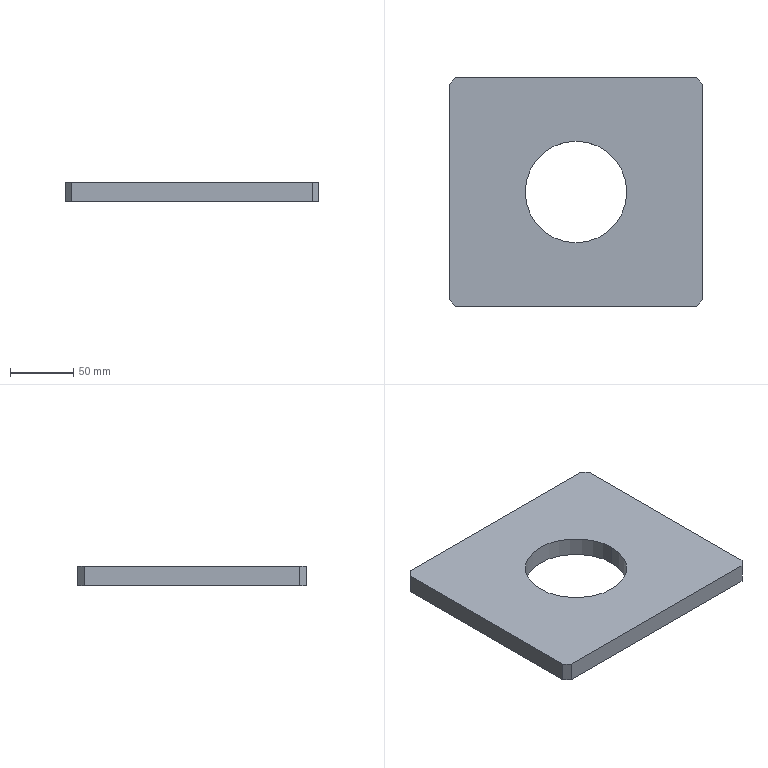Part | STEP file | 001-009-Riveting mechanism electric cylinder spacer block | 1 solid | 12 faces | box 200 x 180 x 15 mm | volume 463852 mm3 | plane 10 | cylinder 2 | commonest cylinder face diameters 80 x2
STEP:
#1=CARTESIAN_POINT('',(0.,0.,0.));
#2=DIRECTION('',(0.,0.,1.));
#3=DIRECTION('',(1.,0.,0.));
#4=AXIS2_PLACEMENT_3D('',#1,#2,#3);
#5=CARTESIAN_POINT('',(40.,0.,0.));
#6=VERTEX_POINT('',#5);
#7=CARTESIAN_POINT('',(40.,0.,15.));
#8=VERTEX_POINT('',#7);
#9=CARTESIAN_POINT('',(40.,0.,0.));
#10=DIRECTION('',(0.,0.,1.));
#11=VECTOR('',#10,1.);
#12=LINE('',#9,#11);
#13=CARTESIAN_POINT('',(0.,0.,0.));
#14=DIRECTION('',(0.,0.,1.));
#15=DIRECTION('',(1.,0.,0.));
#16=AXIS2_PLACEMENT_3D('',#13,#14,#15);
#17=CYLINDRICAL_SURFACE('',#16,40.);
#18=CARTESIAN_POINT('',(6.283,0.));
#19=DIRECTION('',(0.,1.));
#20=VECTOR('',#19,1.);
#21=LINE('',#18,#20);
#22=(GEOMETRIC_REPRESENTATION_CONTEXT(2)PARAMETRIC_REPRESENTATION_CONTEXT()REPRESENTATION_CONTEXT('',''));
#23=DEFINITIONAL_REPRESENTATION('',(#21),#22);
#24=PCURVE('',#17,#23);
#25=CARTESIAN_POINT('',(0.,0.,0.));
#26=DIRECTION('',(0.,0.,1.));
#27=DIRECTION('',(1.,0.,0.));
#28=AXIS2_PLACEMENT_3D('',#25,#26,#27);
#29=CYLINDRICAL_SURFACE('',#28,40.);
#30=CARTESIAN_POINT('',(0.,0.));
#31=DIRECTION('',(0.,1.));
#32=VECTOR('',#31,1.);
#33=LINE('',#30,#32);
#34=(GEOMETRIC_REPRESENTATION_CONTEXT(2)PARAMETRIC_REPRESENTATION_CONTEXT()REPRESENTATION_CONTEXT('',''));
#35=DEFINITIONAL_REPRESENTATION('',(#33),#34);
#36=PCURVE('',#29,#35);
#37=SURFACE_CURVE('',#12,(#24,#36),.PCURVE_S1.);
#38=EDGE_CURVE('',#6,#8,#37,.T.);
#39=ORIENTED_EDGE('',*,*,#38,.T.);
#40=CARTESIAN_POINT('',(-40.,0.,15.));
#41=VERTEX_POINT('',#40);
#42=CARTESIAN_POINT('',(0.,0.,15.));
#43=DIRECTION('',(0.,0.,1.));
#44=DIRECTION('',(1.,0.,0.));
#45=AXIS2_PLACEMENT_3D('',#42,#43,#44);
#46=CIRCLE('',#45,40.);
#47=CARTESIAN_POINT('',(0.,15.));
#48=DIRECTION('',(1.,0.));
#49=VECTOR('',#48,1.);
#50=LINE('',#47,#49);
#51=(GEOMETRIC_REPRESENTATION_CONTEXT(2)PARAMETRIC_REPRESENTATION_CONTEXT()REPRESENTATION_CONTEXT('',''));
#52=DEFINITIONAL_REPRESENTATION('',(#50),#51);
#53=PCURVE('',#17,#52);
#54=CARTESIAN_POINT('',(0.,0.,15.));
#55=DIRECTION('',(0.,0.,-1.));
#56=DIRECTION('',(-1.,0.,0.));
#57=AXIS2_PLACEMENT_3D('',#54,#55,#56);
#58=PLANE('',#57);
#59=CARTESIAN_POINT('',(-40.,0.));
#60=CARTESIAN_POINT('',(-40.,69.282));
#61=CARTESIAN_POINT('',(20.,34.641));
#62=CARTESIAN_POINT('',(80.,0.));
#63=CARTESIAN_POINT('',(20.,-34.641));
#64=CARTESIAN_POINT('',(-40.,-69.282));
#65=CARTESIAN_POINT('',(-40.,0.));
#66=(BOUNDED_CURVE()B_SPLINE_CURVE(2,(#59,#60,#61,#62,#63,#64,#65),.UNSPECIFIED.,.T.,.F.)B_SPLINE_CURVE_WITH_KNOTS((1,2,2,2,2,1),(-2.094,0.,2.094,4.189,6.283,8.378),.UNSPECIFIED.)CURVE()GEOMETRIC_REPRESENTATION_ITEM()RATIONAL_B_SPLINE_CURVE((1.,0.5,1.,0.5,1.,0.5,1.))REPRESENTATION_ITEM(''));
#67=(GEOMETRIC_REPRESENTATION_CONTEXT(2)PARAMETRIC_REPRESENTATION_CONTEXT()REPRESENTATION_CONTEXT('',''));
#68=DEFINITIONAL_REPRESENTATION('',(#66),#67);
#69=PCURVE('',#58,#68);
#70=SURFACE_CURVE('',#46,(#53,#69),.PCURVE_S1.);
#71=EDGE_CURVE('',#41,#8,#70,.T.);
#72=ORIENTED_EDGE('',*,*,#71,.F.);
#73=CARTESIAN_POINT('',(-40.,0.,0.));
#74=VERTEX_POINT('',#73);
#75=CARTESIAN_POINT('',(-40.,0.,0.));
#76=DIRECTION('',(0.,0.,1.));
#77=VECTOR('',#76,1.);
#78=LINE('',#75,#77);
#79=CARTESIAN_POINT('',(3.142,0.));
#80=DIRECTION('',(0.,1.));
#81=VECTOR('',#80,1.);
#82=LINE('',#79,#81);
#83=(GEOMETRIC_REPRESENTATION_CONTEXT(2)PARAMETRIC_REPRESENTATION_CONTEXT()REPRESENTATION_CONTEXT('',''));
#84=DEFINITIONAL_REPRESENTATION('',(#82),#83);
#85=PCURVE('',#17,#84);
#86=CARTESIAN_POINT('',(3.142,0.));
#87=DIRECTION('',(0.,1.));
#88=VECTOR('',#87,1.);
#89=LINE('',#86,#88);
#90=(GEOMETRIC_REPRESENTATION_CONTEXT(2)PARAMETRIC_REPRESENTATION_CONTEXT()REPRESENTATION_CONTEXT('',''));
#91=DEFINITIONAL_REPRESENTATION('',(#89),#90);
#92=PCURVE('',#29,#91);
#93=SURFACE_CURVE('',#78,(#85,#92),.PCURVE_S1.);
#94=EDGE_CURVE('',#74,#41,#93,.T.);
#95=ORIENTED_EDGE('',*,*,#94,.F.);
#96=CARTESIAN_POINT('',(0.,0.,0.));
#97=DIRECTION('',(0.,0.,1.));
#98=DIRECTION('',(1.,0.,0.));
#99=AXIS2_PLACEMENT_3D('',#96,#97,#98);
#100=CIRCLE('',#99,40.);
#101=CARTESIAN_POINT('',(0.,0.));
#102=DIRECTION('',(1.,0.));
#103=VECTOR('',#102,1.);
#104=LINE('',#101,#103);
#105=(GEOMETRIC_REPRESENTATION_CONTEXT(2)PARAMETRIC_REPRESENTATION_CONTEXT()REPRESENTATION_CONTEXT('',''));
#106=DEFINITIONAL_REPRESENTATION('',(#104),#105);
#107=PCURVE('',#17,#106);
#108=CARTESIAN_POINT('',(0.,0.,0.));
#109=DIRECTION('',(0.,0.,-1.));
#110=DIRECTION('',(-1.,0.,0.));
#111=AXIS2_PLACEMENT_3D('',#108,#109,#110);
#112=PLANE('',#111);
#113=CARTESIAN_POINT('',(-40.,0.));
#114=CARTESIAN_POINT('',(-40.,69.282));
#115=CARTESIAN_POINT('',(20.,34.641));
#116=CARTESIAN_POINT('',(80.,0.));
#117=CARTESIAN_POINT('',(20.,-34.641));
#118=CARTESIAN_POINT('',(-40.,-69.282));
#119=CARTESIAN_POINT('',(-40.,0.));
#120=(BOUNDED_CURVE()B_SPLINE_CURVE(2,(#113,#114,#115,#116,#117,#118,#119),.UNSPECIFIED.,.T.,.F.)B_SPLINE_CURVE_WITH_KNOTS((1,2,2,2,2,1),(-2.094,0.,2.094,4.189,6.283,8.378),.UNSPECIFIED.)CURVE()GEOMETRIC_REPRESENTATION_ITEM()RATIONAL_B_SPLINE_CURVE((1.,0.5,1.,0.5,1.,0.5,1.))REPRESENTATION_ITEM(''));
#121=(GEOMETRIC_REPRESENTATION_CONTEXT(2)PARAMETRIC_REPRESENTATION_CONTEXT()REPRESENTATION_CONTEXT('',''));
#122=DEFINITIONAL_REPRESENTATION('',(#120),#121);
#123=PCURVE('',#112,#122);
#124=SURFACE_CURVE('',#100,(#107,#123),.PCURVE_S1.);
#125=EDGE_CURVE('',#74,#6,#124,.T.);
#126=ORIENTED_EDGE('',*,*,#125,.T.);
#127=EDGE_LOOP('',(#39,#72,#95,#126));
#128=FACE_BOUND('',#127,.F.);
#129=ADVANCED_FACE('',(#128),#17,.F.);
#130=CARTESIAN_POINT('',(100.,-85.,15.));
#131=VERTEX_POINT('',#130);
#132=CARTESIAN_POINT('',(100.,85.,15.));
#133=VERTEX_POINT('',#132);
#134=CARTESIAN_POINT('',(100.,-90.,15.));
#135=DIRECTION('',(0.,1.,0.));
#136=VECTOR('',#135,1.);
#137=LINE('',#134,#136);
#138=CARTESIAN_POINT('',(100.,-90.,15.));
#139=DIRECTION('',(-1.,0.,0.));
#140=DIRECTION('',(0.,-1.,0.));
#141=AXIS2_PLACEMENT_3D('',#138,#139,#140);
#142=PLANE('',#141);
#143=CARTESIAN_POINT('',(0.,0.));
#144=DIRECTION('',(-1.,0.));
#145=VECTOR('',#144,1.);
#146=LINE('',#143,#145);
#147=(GEOMETRIC_REPRESENTATION_CONTEXT(2)PARAMETRIC_REPRESENTATION_CONTEXT()REPRESENTATION_CONTEXT('',''));
#148=DEFINITIONAL_REPRESENTATION('',(#146),#147);
#149=PCURVE('',#142,#148);
#150=CARTESIAN_POINT('',(-100.,-90.));
#151=DIRECTION('',(0.,1.));
#152=VECTOR('',#151,1.);
#153=LINE('',#150,#152);
#154=(GEOMETRIC_REPRESENTATION_CONTEXT(2)PARAMETRIC_REPRESENTATION_CONTEXT()REPRESENTATION_CONTEXT('',''));
#155=DEFINITIONAL_REPRESENTATION('',(#153),#154);
#156=PCURVE('',#58,#155);
#157=SURFACE_CURVE('',#137,(#149,#156),.PCURVE_S1.);
#158=EDGE_CURVE('',#131,#133,#157,.T.);
#159=ORIENTED_EDGE('',*,*,#158,.F.);
#160=CARTESIAN_POINT('',(100.,-85.,0.));
#161=VERTEX_POINT('',#160);
#162=CARTESIAN_POINT('',(100.,-85.,15.));
#163=DIRECTION('',(0.,0.,-1.));
#164=VECTOR('',#163,1.);
#165=LINE('',#162,#164);
#166=CARTESIAN_POINT('',(-5.,0.));
#167=DIRECTION('',(0.,-1.));
#168=VECTOR('',#167,1.);
#169=LINE('',#166,#168);
#170=(GEOMETRIC_REPRESENTATION_CONTEXT(2)PARAMETRIC_REPRESENTATION_CONTEXT()REPRESENTATION_CONTEXT('',''));
#171=DEFINITIONAL_REPRESENTATION('',(#169),#170);
#172=PCURVE('',#142,#171);
#173=CARTESIAN_POINT('',(100.,-85.,15.));
#174=DIRECTION('',(-0.7071,0.7071,0.));
#175=DIRECTION('',(0.,0.,-1.));
#176=AXIS2_PLACEMENT_3D('',#173,#174,#175);
#177=PLANE('',#176);
#178=CARTESIAN_POINT('',(0.,0.));
#179=DIRECTION('',(1.,0.));
#180=VECTOR('',#179,1.);
#181=LINE('',#178,#180);
#182=(GEOMETRIC_REPRESENTATION_CONTEXT(2)PARAMETRIC_REPRESENTATION_CONTEXT()REPRESENTATION_CONTEXT('',''));
#183=DEFINITIONAL_REPRESENTATION('',(#181),#182);
#184=PCURVE('',#177,#183);
#185=SURFACE_CURVE('',#165,(#172,#184),.PCURVE_S1.);
#186=EDGE_CURVE('',#131,#161,#185,.T.);
#187=ORIENTED_EDGE('',*,*,#186,.T.);
#188=CARTESIAN_POINT('',(100.,85.,0.));
#189=VERTEX_POINT('',#188);
#190=CARTESIAN_POINT('',(100.,-90.,0.));
#191=DIRECTION('',(0.,1.,0.));
#192=VECTOR('',#191,1.);
#193=LINE('',#190,#192);
#194=CARTESIAN_POINT('',(0.,-15.));
#195=DIRECTION('',(-1.,0.));
#196=VECTOR('',#195,1.);
#197=LINE('',#194,#196);
#198=(GEOMETRIC_REPRESENTATION_CONTEXT(2)PARAMETRIC_REPRESENTATION_CONTEXT()REPRESENTATION_CONTEXT('',''));
#199=DEFINITIONAL_REPRESENTATION('',(#197),#198);
#200=PCURVE('',#142,#199);
#201=CARTESIAN_POINT('',(-100.,-90.));
#202=DIRECTION('',(0.,1.));
#203=VECTOR('',#202,1.);
#204=LINE('',#201,#203);
#205=(GEOMETRIC_REPRESENTATION_CONTEXT(2)PARAMETRIC_REPRESENTATION_CONTEXT()REPRESENTATION_CONTEXT('',''));
#206=DEFINITIONAL_REPRESENTATION('',(#204),#205);
#207=PCURVE('',#112,#206);
#208=SURFACE_CURVE('',#193,(#200,#207),.PCURVE_S1.);
#209=EDGE_CURVE('',#161,#189,#208,.T.);
#210=ORIENTED_EDGE('',*,*,#209,.T.);
#211=CARTESIAN_POINT('',(100.,85.,15.));
#212=DIRECTION('',(0.,0.,1.));
#213=VECTOR('',#212,1.);
#214=LINE('',#211,#213);
#215=CARTESIAN_POINT('',(-175.,0.));
#216=DIRECTION('',(0.,1.));
#217=VECTOR('',#216,1.);
#218=LINE('',#215,#217);
#219=(GEOMETRIC_REPRESENTATION_CONTEXT(2)PARAMETRIC_REPRESENTATION_CONTEXT()REPRESENTATION_CONTEXT('',''));
#220=DEFINITIONAL_REPRESENTATION('',(#218),#219);
#221=PCURVE('',#142,#220);
#222=CARTESIAN_POINT('',(95.,90.,15.));
#223=DIRECTION('',(-0.7071,-0.7071,0.));
#224=DIRECTION('',(0.,0.,-1.));
#225=AXIS2_PLACEMENT_3D('',#222,#223,#224);
#226=PLANE('',#225);
#227=CARTESIAN_POINT('',(0.,7.071));
#228=DIRECTION('',(-1.,0.));
#229=VECTOR('',#228,1.);
#230=LINE('',#227,#229);
#231=(GEOMETRIC_REPRESENTATION_CONTEXT(2)PARAMETRIC_REPRESENTATION_CONTEXT()REPRESENTATION_CONTEXT('',''));
#232=DEFINITIONAL_REPRESENTATION('',(#230),#231);
#233=PCURVE('',#226,#232);
#234=SURFACE_CURVE('',#214,(#221,#233),.PCURVE_S1.);
#235=EDGE_CURVE('',#189,#133,#234,.T.);
#236=ORIENTED_EDGE('',*,*,#235,.T.);
#237=EDGE_LOOP('',(#159,#187,#210,#236));
#238=FACE_BOUND('',#237,.T.);
#239=ADVANCED_FACE('',(#238),#142,.F.);
#240=CARTESIAN_POINT('',(95.,90.,0.));
#241=VERTEX_POINT('',#240);
#242=CARTESIAN_POINT('',(-95.,90.,0.));
#243=VERTEX_POINT('',#242);
#244=CARTESIAN_POINT('',(-100.,90.,0.));
#245=DIRECTION('',(-1.,0.,0.));
#246=VECTOR('',#245,1.);
#247=LINE('',#244,#246);
#248=CARTESIAN_POINT('',(-100.,90.,15.));
#249=DIRECTION('',(0.,-1.,0.));
#250=DIRECTION('',(0.,0.,-1.));
#251=AXIS2_PLACEMENT_3D('',#248,#249,#250);
#252=PLANE('',#251);
#253=CARTESIAN_POINT('',(15.,0.));
#254=DIRECTION('',(0.,-1.));
#255=VECTOR('',#254,1.);
#256=LINE('',#253,#255);
#257=(GEOMETRIC_REPRESENTATION_CONTEXT(2)PARAMETRIC_REPRESENTATION_CONTEXT()REPRESENTATION_CONTEXT('',''));
#258=DEFINITIONAL_REPRESENTATION('',(#256),#257);
#259=PCURVE('',#252,#258);
#260=CARTESIAN_POINT('',(100.,90.));
#261=DIRECTION('',(1.,0.));
#262=VECTOR('',#261,1.);
#263=LINE('',#260,#262);
#264=(GEOMETRIC_REPRESENTATION_CONTEXT(2)PARAMETRIC_REPRESENTATION_CONTEXT()REPRESENTATION_CONTEXT('',''));
#265=DEFINITIONAL_REPRESENTATION('',(#263),#264);
#266=PCURVE('',#112,#265);
#267=SURFACE_CURVE('',#247,(#259,#266),.PCURVE_S1.);
#268=EDGE_CURVE('',#241,#243,#267,.T.);
#269=ORIENTED_EDGE('',*,*,#268,.T.);
#270=CARTESIAN_POINT('',(-95.,90.,15.));
#271=VERTEX_POINT('',#270);
#272=CARTESIAN_POINT('',(-95.,90.,15.));
#273=DIRECTION('',(0.,0.,1.));
#274=VECTOR('',#273,1.);
#275=LINE('',#272,#274);
#276=CARTESIAN_POINT('',(0.,5.));
#277=DIRECTION('',(-1.,0.));
#278=VECTOR('',#277,1.);
#279=LINE('',#276,#278);
#280=(GEOMETRIC_REPRESENTATION_CONTEXT(2)PARAMETRIC_REPRESENTATION_CONTEXT()REPRESENTATION_CONTEXT('',''));
#281=DEFINITIONAL_REPRESENTATION('',(#279),#280);
#282=PCURVE('',#252,#281);
#283=CARTESIAN_POINT('',(-100.,85.,15.));
#284=DIRECTION('',(0.7071,-0.7071,0.));
#285=DIRECTION('',(0.,0.,-1.));
#286=AXIS2_PLACEMENT_3D('',#283,#284,#285);
#287=PLANE('',#286);
#288=CARTESIAN_POINT('',(0.,7.071));
#289=DIRECTION('',(-1.,0.));
#290=VECTOR('',#289,1.);
#291=LINE('',#288,#290);
#292=(GEOMETRIC_REPRESENTATION_CONTEXT(2)PARAMETRIC_REPRESENTATION_CONTEXT()REPRESENTATION_CONTEXT('',''));
#293=DEFINITIONAL_REPRESENTATION('',(#291),#292);
#294=PCURVE('',#287,#293);
#295=SURFACE_CURVE('',#275,(#282,#294),.PCURVE_S1.);
#296=EDGE_CURVE('',#243,#271,#295,.T.);
#297=ORIENTED_EDGE('',*,*,#296,.T.);
#298=CARTESIAN_POINT('',(95.,90.,15.));
#299=VERTEX_POINT('',#298);
#300=CARTESIAN_POINT('',(-100.,90.,15.));
#301=DIRECTION('',(-1.,0.,0.));
#302=VECTOR('',#301,1.);
#303=LINE('',#300,#302);
#304=CARTESIAN_POINT('',(0.,0.));
#305=DIRECTION('',(0.,-1.));
#306=VECTOR('',#305,1.);
#307=LINE('',#304,#306);
#308=(GEOMETRIC_REPRESENTATION_CONTEXT(2)PARAMETRIC_REPRESENTATION_CONTEXT()REPRESENTATION_CONTEXT('',''));
#309=DEFINITIONAL_REPRESENTATION('',(#307),#308);
#310=PCURVE('',#252,#309);
#311=CARTESIAN_POINT('',(100.,90.));
#312=DIRECTION('',(1.,0.));
#313=VECTOR('',#312,1.);
#314=LINE('',#311,#313);
#315=(GEOMETRIC_REPRESENTATION_CONTEXT(2)PARAMETRIC_REPRESENTATION_CONTEXT()REPRESENTATION_CONTEXT('',''));
#316=DEFINITIONAL_REPRESENTATION('',(#314),#315);
#317=PCURVE('',#58,#316);
#318=SURFACE_CURVE('',#303,(#310,#317),.PCURVE_S1.);
#319=EDGE_CURVE('',#299,#271,#318,.T.);
#320=ORIENTED_EDGE('',*,*,#319,.F.);
#321=CARTESIAN_POINT('',(95.,90.,15.));
#322=DIRECTION('',(0.,0.,-1.));
#323=VECTOR('',#322,1.);
#324=LINE('',#321,#323);
#325=CARTESIAN_POINT('',(0.,195.));
#326=DIRECTION('',(1.,0.));
#327=VECTOR('',#326,1.);
#328=LINE('',#325,#327);
#329=(GEOMETRIC_REPRESENTATION_CONTEXT(2)PARAMETRIC_REPRESENTATION_CONTEXT()REPRESENTATION_CONTEXT('',''));
#330=DEFINITIONAL_REPRESENTATION('',(#328),#329);
#331=PCURVE('',#252,#330);
#332=CARTESIAN_POINT('',(0.,0.));
#333=DIRECTION('',(1.,0.));
#334=VECTOR('',#333,1.);
#335=LINE('',#332,#334);
#336=(GEOMETRIC_REPRESENTATION_CONTEXT(2)PARAMETRIC_REPRESENTATION_CONTEXT()REPRESENTATION_CONTEXT('',''));
#337=DEFINITIONAL_REPRESENTATION('',(#335),#336);
#338=PCURVE('',#226,#337);
#339=SURFACE_CURVE('',#324,(#331,#338),.PCURVE_S1.);
#340=EDGE_CURVE('',#299,#241,#339,.T.);
#341=ORIENTED_EDGE('',*,*,#340,.T.);
#342=EDGE_LOOP('',(#269,#297,#320,#341));
#343=FACE_BOUND('',#342,.T.);
#344=ADVANCED_FACE('',(#343),#252,.F.);
#345=CARTESIAN_POINT('',(-100.,85.,0.));
#346=VERTEX_POINT('',#345);
#347=CARTESIAN_POINT('',(-100.,-85.,0.));
#348=VERTEX_POINT('',#347);
#349=CARTESIAN_POINT('',(-100.,-90.,0.));
#350=DIRECTION('',(0.,-1.,0.));
#351=VECTOR('',#350,1.);
#352=LINE('',#349,#351);
#353=CARTESIAN_POINT('',(-100.,-90.,15.));
#354=DIRECTION('',(1.,0.,0.));
#355=DIRECTION('',(0.,0.,-1.));
#356=AXIS2_PLACEMENT_3D('',#353,#354,#355);
#357=PLANE('',#356);
#358=CARTESIAN_POINT('',(15.,0.));
#359=DIRECTION('',(0.,-1.));
#360=VECTOR('',#359,1.);
#361=LINE('',#358,#360);
#362=(GEOMETRIC_REPRESENTATION_CONTEXT(2)PARAMETRIC_REPRESENTATION_CONTEXT()REPRESENTATION_CONTEXT('',''));
#363=DEFINITIONAL_REPRESENTATION('',(#361),#362);
#364=PCURVE('',#357,#363);
#365=CARTESIAN_POINT('',(100.,-90.));
#366=DIRECTION('',(0.,-1.));
#367=VECTOR('',#366,1.);
#368=LINE('',#365,#367);
#369=(GEOMETRIC_REPRESENTATION_CONTEXT(2)PARAMETRIC_REPRESENTATION_CONTEXT()REPRESENTATION_CONTEXT('',''));
#370=DEFINITIONAL_REPRESENTATION('',(#368),#369);
#371=PCURVE('',#112,#370);
#372=SURFACE_CURVE('',#352,(#364,#371),.PCURVE_S1.);
#373=EDGE_CURVE('',#346,#348,#372,.T.);
#374=ORIENTED_EDGE('',*,*,#373,.T.);
#375=CARTESIAN_POINT('',(-100.,-85.,15.));
#376=VERTEX_POINT('',#375);
#377=CARTESIAN_POINT('',(-100.,-85.,15.));
#378=DIRECTION('',(0.,0.,1.));
#379=VECTOR('',#378,1.);
#380=LINE('',#377,#379);
#381=CARTESIAN_POINT('',(0.,5.));
#382=DIRECTION('',(-1.,0.));
#383=VECTOR('',#382,1.);
#384=LINE('',#381,#383);
#385=(GEOMETRIC_REPRESENTATION_CONTEXT(2)PARAMETRIC_REPRESENTATION_CONTEXT()REPRESENTATION_CONTEXT('',''));
#386=DEFINITIONAL_REPRESENTATION('',(#384),#385);
#387=PCURVE('',#357,#386);
#388=CARTESIAN_POINT('',(-95.,-90.,15.));
#389=DIRECTION('',(0.7071,0.7071,0.));
#390=DIRECTION('',(0.,0.,-1.));
#391=AXIS2_PLACEMENT_3D('',#388,#389,#390);
#392=PLANE('',#391);
#393=CARTESIAN_POINT('',(0.,7.071));
#394=DIRECTION('',(-1.,0.));
#395=VECTOR('',#394,1.);
#396=LINE('',#393,#395);
#397=(GEOMETRIC_REPRESENTATION_CONTEXT(2)PARAMETRIC_REPRESENTATION_CONTEXT()REPRESENTATION_CONTEXT('',''));
#398=DEFINITIONAL_REPRESENTATION('',(#396),#397);
#399=PCURVE('',#392,#398);
#400=SURFACE_CURVE('',#380,(#387,#399),.PCURVE_S1.);
#401=EDGE_CURVE('',#348,#376,#400,.T.);
#402=ORIENTED_EDGE('',*,*,#401,.T.);
#403=CARTESIAN_POINT('',(-100.,85.,15.));
#404=VERTEX_POINT('',#403);
#405=CARTESIAN_POINT('',(-100.,-90.,15.));
#406=DIRECTION('',(0.,-1.,0.));
#407=VECTOR('',#406,1.);
#408=LINE('',#405,#407);
#409=CARTESIAN_POINT('',(0.,0.));
#410=DIRECTION('',(0.,-1.));
#411=VECTOR('',#410,1.);
#412=LINE('',#409,#411);
#413=(GEOMETRIC_REPRESENTATION_CONTEXT(2)PARAMETRIC_REPRESENTATION_CONTEXT()REPRESENTATION_CONTEXT('',''));
#414=DEFINITIONAL_REPRESENTATION('',(#412),#413);
#415=PCURVE('',#357,#414);
#416=CARTESIAN_POINT('',(100.,-90.));
#417=DIRECTION('',(0.,-1.));
#418=VECTOR('',#417,1.);
#419=LINE('',#416,#418);
#420=(GEOMETRIC_REPRESENTATION_CONTEXT(2)PARAMETRIC_REPRESENTATION_CONTEXT()REPRESENTATION_CONTEXT('',''));
#421=DEFINITIONAL_REPRESENTATION('',(#419),#420);
#422=PCURVE('',#58,#421);
#423=SURFACE_CURVE('',#408,(#415,#422),.PCURVE_S1.);
#424=EDGE_CURVE('',#404,#376,#423,.T.);
#425=ORIENTED_EDGE('',*,*,#424,.F.);
#426=CARTESIAN_POINT('',(-100.,85.,15.));
#427=DIRECTION('',(0.,0.,-1.));
#428=VECTOR('',#427,1.);
#429=LINE('',#426,#428);
#430=CARTESIAN_POINT('',(0.,175.));
#431=DIRECTION('',(1.,0.));
#432=VECTOR('',#431,1.);
#433=LINE('',#430,#432);
#434=(GEOMETRIC_REPRESENTATION_CONTEXT(2)PARAMETRIC_REPRESENTATION_CONTEXT()REPRESENTATION_CONTEXT('',''));
#435=DEFINITIONAL_REPRESENTATION('',(#433),#434);
#436=PCURVE('',#357,#435);
#437=CARTESIAN_POINT('',(0.,0.));
#438=DIRECTION('',(1.,0.));
#439=VECTOR('',#438,1.);
#440=LINE('',#437,#439);
#441=(GEOMETRIC_REPRESENTATION_CONTEXT(2)PARAMETRIC_REPRESENTATION_CONTEXT()REPRESENTATION_CONTEXT('',''));
#442=DEFINITIONAL_REPRESENTATION('',(#440),#441);
#443=PCURVE('',#287,#442);
#444=SURFACE_CURVE('',#429,(#436,#443),.PCURVE_S1.);
#445=EDGE_CURVE('',#404,#346,#444,.T.);
#446=ORIENTED_EDGE('',*,*,#445,.T.);
#447=EDGE_LOOP('',(#374,#402,#425,#446));
#448=FACE_BOUND('',#447,.T.);
#449=ADVANCED_FACE('',(#448),#357,.F.);
#450=CARTESIAN_POINT('',(-95.,-90.,0.));
#451=VERTEX_POINT('',#450);
#452=CARTESIAN_POINT('',(95.,-90.,0.));
#453=VERTEX_POINT('',#452);
#454=CARTESIAN_POINT('',(-100.,-90.,0.));
#455=DIRECTION('',(1.,0.,0.));
#456=VECTOR('',#455,1.);
#457=LINE('',#454,#456);
#458=CARTESIAN_POINT('',(-100.,-90.,15.));
#459=DIRECTION('',(0.,1.,0.));
#460=DIRECTION('',(0.,0.,1.));
#461=AXIS2_PLACEMENT_3D('',#458,#459,#460);
#462=PLANE('',#461);
#463=CARTESIAN_POINT('',(-15.,0.));
#464=DIRECTION('',(0.,1.));
#465=VECTOR('',#464,1.);
#466=LINE('',#463,#465);
#467=(GEOMETRIC_REPRESENTATION_CONTEXT(2)PARAMETRIC_REPRESENTATION_CONTEXT()REPRESENTATION_CONTEXT('',''));
#468=DEFINITIONAL_REPRESENTATION('',(#466),#467);
#469=PCURVE('',#462,#468);
#470=CARTESIAN_POINT('',(100.,-90.));
#471=DIRECTION('',(-1.,0.));
#472=VECTOR('',#471,1.);
#473=LINE('',#470,#472);
#474=(GEOMETRIC_REPRESENTATION_CONTEXT(2)PARAMETRIC_REPRESENTATION_CONTEXT()REPRESENTATION_CONTEXT('',''));
#475=DEFINITIONAL_REPRESENTATION('',(#473),#474);
#476=PCURVE('',#112,#475);
#477=SURFACE_CURVE('',#457,(#469,#476),.PCURVE_S1.);
#478=EDGE_CURVE('',#451,#453,#477,.T.);
#479=ORIENTED_EDGE('',*,*,#478,.T.);
#480=CARTESIAN_POINT('',(95.,-90.,15.));
#481=VERTEX_POINT('',#480);
#482=CARTESIAN_POINT('',(95.,-90.,15.));
#483=DIRECTION('',(0.,0.,1.));
#484=VECTOR('',#483,1.);
#485=LINE('',#482,#484);
#486=CARTESIAN_POINT('',(0.,195.));
#487=DIRECTION('',(1.,0.));
#488=VECTOR('',#487,1.);
#489=LINE('',#486,#488);
#490=(GEOMETRIC_REPRESENTATION_CONTEXT(2)PARAMETRIC_REPRESENTATION_CONTEXT()REPRESENTATION_CONTEXT('',''));
#491=DEFINITIONAL_REPRESENTATION('',(#489),#490);
#492=PCURVE('',#462,#491);
#493=CARTESIAN_POINT('',(0.,7.071));
#494=DIRECTION('',(-1.,0.));
#495=VECTOR('',#494,1.);
#496=LINE('',#493,#495);
#497=(GEOMETRIC_REPRESENTATION_CONTEXT(2)PARAMETRIC_REPRESENTATION_CONTEXT()REPRESENTATION_CONTEXT('',''));
#498=DEFINITIONAL_REPRESENTATION('',(#496),#497);
#499=PCURVE('',#177,#498);
#500=SURFACE_CURVE('',#485,(#492,#499),.PCURVE_S1.);
#501=EDGE_CURVE('',#453,#481,#500,.T.);
#502=ORIENTED_EDGE('',*,*,#501,.T.);
#503=CARTESIAN_POINT('',(-95.,-90.,15.));
#504=VERTEX_POINT('',#503);
#505=CARTESIAN_POINT('',(-100.,-90.,15.));
#506=DIRECTION('',(1.,0.,0.));
#507=VECTOR('',#506,1.);
#508=LINE('',#505,#507);
#509=CARTESIAN_POINT('',(0.,0.));
#510=DIRECTION('',(0.,1.));
#511=VECTOR('',#510,1.);
#512=LINE('',#509,#511);
#513=(GEOMETRIC_REPRESENTATION_CONTEXT(2)PARAMETRIC_REPRESENTATION_CONTEXT()REPRESENTATION_CONTEXT('',''));
#514=DEFINITIONAL_REPRESENTATION('',(#512),#513);
#515=PCURVE('',#462,#514);
#516=CARTESIAN_POINT('',(100.,-90.));
#517=DIRECTION('',(-1.,0.));
#518=VECTOR('',#517,1.);
#519=LINE('',#516,#518);
#520=(GEOMETRIC_REPRESENTATION_CONTEXT(2)PARAMETRIC_REPRESENTATION_CONTEXT()REPRESENTATION_CONTEXT('',''));
#521=DEFINITIONAL_REPRESENTATION('',(#519),#520);
#522=PCURVE('',#58,#521);
#523=SURFACE_CURVE('',#508,(#515,#522),.PCURVE_S1.);
#524=EDGE_CURVE('',#504,#481,#523,.T.);
#525=ORIENTED_EDGE('',*,*,#524,.F.);
#526=CARTESIAN_POINT('',(-95.,-90.,15.));
#527=DIRECTION('',(0.,0.,-1.));
#528=VECTOR('',#527,1.);
#529=LINE('',#526,#528);
#530=CARTESIAN_POINT('',(0.,5.));
#531=DIRECTION('',(-1.,0.));
#532=VECTOR('',#531,1.);
#533=LINE('',#530,#532);
#534=(GEOMETRIC_REPRESENTATION_CONTEXT(2)PARAMETRIC_REPRESENTATION_CONTEXT()REPRESENTATION_CONTEXT('',''));
#535=DEFINITIONAL_REPRESENTATION('',(#533),#534);
#536=PCURVE('',#462,#535);
#537=CARTESIAN_POINT('',(0.,0.));
#538=DIRECTION('',(1.,0.));
#539=VECTOR('',#538,1.);
#540=LINE('',#537,#539);
#541=(GEOMETRIC_REPRESENTATION_CONTEXT(2)PARAMETRIC_REPRESENTATION_CONTEXT()REPRESENTATION_CONTEXT('',''));
#542=DEFINITIONAL_REPRESENTATION('',(#540),#541);
#543=PCURVE('',#392,#542);
#544=SURFACE_CURVE('',#529,(#536,#543),.PCURVE_S1.);
#545=EDGE_CURVE('',#504,#451,#544,.T.);
#546=ORIENTED_EDGE('',*,*,#545,.T.);
#547=EDGE_LOOP('',(#479,#502,#525,#546));
#548=FACE_BOUND('',#547,.T.);
#549=ADVANCED_FACE('',(#548),#462,.F.);
#550=CARTESIAN_POINT('',(0.,0.,15.));
#551=DIRECTION('',(0.,0.,1.));
#552=DIRECTION('',(1.,0.,0.));
#553=AXIS2_PLACEMENT_3D('',#550,#551,#552);
#554=CIRCLE('',#553,40.);
#555=CARTESIAN_POINT('',(-40.,0.));
#556=CARTESIAN_POINT('',(-40.,69.282));
#557=CARTESIAN_POINT('',(20.,34.641));
#558=CARTESIAN_POINT('',(80.,0.));
#559=CARTESIAN_POINT('',(20.,-34.641));
#560=CARTESIAN_POINT('',(-40.,-69.282));
#561=CARTESIAN_POINT('',(-40.,0.));
#562=(BOUNDED_CURVE()B_SPLINE_CURVE(2,(#555,#556,#557,#558,#559,#560,#561),.UNSPECIFIED.,.T.,.F.)B_SPLINE_CURVE_WITH_KNOTS((1,2,2,2,2,1),(-2.094,0.,2.094,4.189,6.283,8.378),.UNSPECIFIED.)CURVE()GEOMETRIC_REPRESENTATION_ITEM()RATIONAL_B_SPLINE_CURVE((1.,0.5,1.,0.5,1.,0.5,1.))REPRESENTATION_ITEM(''));
#563=(GEOMETRIC_REPRESENTATION_CONTEXT(2)PARAMETRIC_REPRESENTATION_CONTEXT()REPRESENTATION_CONTEXT('',''));
#564=DEFINITIONAL_REPRESENTATION('',(#562),#563);
#565=PCURVE('',#58,#564);
#566=CARTESIAN_POINT('',(0.,15.));
#567=DIRECTION('',(1.,0.));
#568=VECTOR('',#567,1.);
#569=LINE('',#566,#568);
#570=(GEOMETRIC_REPRESENTATION_CONTEXT(2)PARAMETRIC_REPRESENTATION_CONTEXT()REPRESENTATION_CONTEXT('',''));
#571=DEFINITIONAL_REPRESENTATION('',(#569),#570);
#572=PCURVE('',#29,#571);
#573=SURFACE_CURVE('',#554,(#565,#572),.PCURVE_S1.);
#574=EDGE_CURVE('',#8,#41,#573,.T.);
#575=ORIENTED_EDGE('',*,*,#574,.F.);
#576=ORIENTED_EDGE('',*,*,#71,.F.);
#577=EDGE_LOOP('',(#575,#576));
#578=FACE_BOUND('',#577,.T.);
#579=ORIENTED_EDGE('',*,*,#524,.T.);
#580=CARTESIAN_POINT('',(100.,-85.,15.));
#581=DIRECTION('',(0.7071,0.7071,0.));
#582=VECTOR('',#581,1.);
#583=LINE('',#580,#582);
#584=CARTESIAN_POINT('',(-100.,-85.));
#585=DIRECTION('',(-0.7071,0.7071));
#586=VECTOR('',#585,1.);
#587=LINE('',#584,#586);
#588=(GEOMETRIC_REPRESENTATION_CONTEXT(2)PARAMETRIC_REPRESENTATION_CONTEXT()REPRESENTATION_CONTEXT('',''));
#589=DEFINITIONAL_REPRESENTATION('',(#587),#588);
#590=PCURVE('',#58,#589);
#591=CARTESIAN_POINT('',(0.,0.));
#592=DIRECTION('',(0.,-1.));
#593=VECTOR('',#592,1.);
#594=LINE('',#591,#593);
#595=(GEOMETRIC_REPRESENTATION_CONTEXT(2)PARAMETRIC_REPRESENTATION_CONTEXT()REPRESENTATION_CONTEXT('',''));
#596=DEFINITIONAL_REPRESENTATION('',(#594),#595);
#597=PCURVE('',#177,#596);
#598=SURFACE_CURVE('',#583,(#590,#597),.PCURVE_S1.);
#599=EDGE_CURVE('',#481,#131,#598,.T.);
#600=ORIENTED_EDGE('',*,*,#599,.T.);
#601=ORIENTED_EDGE('',*,*,#158,.T.);
#602=CARTESIAN_POINT('',(95.,90.,15.));
#603=DIRECTION('',(-0.7071,0.7071,0.));
#604=VECTOR('',#603,1.);
#605=LINE('',#602,#604);
#606=CARTESIAN_POINT('',(-95.,90.));
#607=DIRECTION('',(0.7071,0.7071));
#608=VECTOR('',#607,1.);
#609=LINE('',#606,#608);
#610=(GEOMETRIC_REPRESENTATION_CONTEXT(2)PARAMETRIC_REPRESENTATION_CONTEXT()REPRESENTATION_CONTEXT('',''));
#611=DEFINITIONAL_REPRESENTATION('',(#609),#610);
#612=PCURVE('',#58,#611);
#613=CARTESIAN_POINT('',(0.,0.));
#614=DIRECTION('',(0.,-1.));
#615=VECTOR('',#614,1.);
#616=LINE('',#613,#615);
#617=(GEOMETRIC_REPRESENTATION_CONTEXT(2)PARAMETRIC_REPRESENTATION_CONTEXT()REPRESENTATION_CONTEXT('',''));
#618=DEFINITIONAL_REPRESENTATION('',(#616),#617);
#619=PCURVE('',#226,#618);
#620=SURFACE_CURVE('',#605,(#612,#619),.PCURVE_S1.);
#621=EDGE_CURVE('',#133,#299,#620,.T.);
#622=ORIENTED_EDGE('',*,*,#621,.T.);
#623=ORIENTED_EDGE('',*,*,#319,.T.);
#624=CARTESIAN_POINT('',(-100.,85.,15.));
#625=DIRECTION('',(-0.7071,-0.7071,0.));
#626=VECTOR('',#625,1.);
#627=LINE('',#624,#626);
#628=CARTESIAN_POINT('',(100.,85.));
#629=DIRECTION('',(0.7071,-0.7071));
#630=VECTOR('',#629,1.);
#631=LINE('',#628,#630);
#632=(GEOMETRIC_REPRESENTATION_CONTEXT(2)PARAMETRIC_REPRESENTATION_CONTEXT()REPRESENTATION_CONTEXT('',''));
#633=DEFINITIONAL_REPRESENTATION('',(#631),#632);
#634=PCURVE('',#58,#633);
#635=CARTESIAN_POINT('',(0.,0.));
#636=DIRECTION('',(0.,-1.));
#637=VECTOR('',#636,1.);
#638=LINE('',#635,#637);
#639=(GEOMETRIC_REPRESENTATION_CONTEXT(2)PARAMETRIC_REPRESENTATION_CONTEXT()REPRESENTATION_CONTEXT('',''));
#640=DEFINITIONAL_REPRESENTATION('',(#638),#639);
#641=PCURVE('',#287,#640);
#642=SURFACE_CURVE('',#627,(#634,#641),.PCURVE_S1.);
#643=EDGE_CURVE('',#271,#404,#642,.T.);
#644=ORIENTED_EDGE('',*,*,#643,.T.);
#645=ORIENTED_EDGE('',*,*,#424,.T.);
#646=CARTESIAN_POINT('',(-95.,-90.,15.));
#647=DIRECTION('',(0.7071,-0.7071,0.));
#648=VECTOR('',#647,1.);
#649=LINE('',#646,#648);
#650=CARTESIAN_POINT('',(95.,-90.));
#651=DIRECTION('',(-0.7071,-0.7071));
#652=VECTOR('',#651,1.);
#653=LINE('',#650,#652);
#654=(GEOMETRIC_REPRESENTATION_CONTEXT(2)PARAMETRIC_REPRESENTATION_CONTEXT()REPRESENTATION_CONTEXT('',''));
#655=DEFINITIONAL_REPRESENTATION('',(#653),#654);
#656=PCURVE('',#58,#655);
#657=CARTESIAN_POINT('',(0.,0.));
#658=DIRECTION('',(0.,-1.));
#659=VECTOR('',#658,1.);
#660=LINE('',#657,#659);
#661=(GEOMETRIC_REPRESENTATION_CONTEXT(2)PARAMETRIC_REPRESENTATION_CONTEXT()REPRESENTATION_CONTEXT('',''));
#662=DEFINITIONAL_REPRESENTATION('',(#660),#661);
#663=PCURVE('',#392,#662);
#664=SURFACE_CURVE('',#649,(#656,#663),.PCURVE_S1.);
#665=EDGE_CURVE('',#376,#504,#664,.T.);
#666=ORIENTED_EDGE('',*,*,#665,.T.);
#667=EDGE_LOOP('',(#579,#600,#601,#622,#623,#644,#645,#666));
#668=FACE_BOUND('',#667,.T.);
#669=ADVANCED_FACE('',(#578,#668),#58,.F.);
#670=CARTESIAN_POINT('',(0.,0.,0.));
#671=DIRECTION('',(0.,0.,1.));
#672=DIRECTION('',(1.,0.,0.));
#673=AXIS2_PLACEMENT_3D('',#670,#671,#672);
#674=CIRCLE('',#673,40.);
#675=CARTESIAN_POINT('',(-40.,0.));
#676=CARTESIAN_POINT('',(-40.,69.282));
#677=CARTESIAN_POINT('',(20.,34.641));
#678=CARTESIAN_POINT('',(80.,0.));
#679=CARTESIAN_POINT('',(20.,-34.641));
#680=CARTESIAN_POINT('',(-40.,-69.282));
#681=CARTESIAN_POINT('',(-40.,0.));
#682=(BOUNDED_CURVE()B_SPLINE_CURVE(2,(#675,#676,#677,#678,#679,#680,#681),.UNSPECIFIED.,.T.,.F.)B_SPLINE_CURVE_WITH_KNOTS((1,2,2,2,2,1),(-2.094,0.,2.094,4.189,6.283,8.378),.UNSPECIFIED.)CURVE()GEOMETRIC_REPRESENTATION_ITEM()RATIONAL_B_SPLINE_CURVE((1.,0.5,1.,0.5,1.,0.5,1.))REPRESENTATION_ITEM(''));
#683=(GEOMETRIC_REPRESENTATION_CONTEXT(2)PARAMETRIC_REPRESENTATION_CONTEXT()REPRESENTATION_CONTEXT('',''));
#684=DEFINITIONAL_REPRESENTATION('',(#682),#683);
#685=PCURVE('',#112,#684);
#686=CARTESIAN_POINT('',(0.,0.));
#687=DIRECTION('',(1.,0.));
#688=VECTOR('',#687,1.);
#689=LINE('',#686,#688);
#690=(GEOMETRIC_REPRESENTATION_CONTEXT(2)PARAMETRIC_REPRESENTATION_CONTEXT()REPRESENTATION_CONTEXT('',''));
#691=DEFINITIONAL_REPRESENTATION('',(#689),#690);
#692=PCURVE('',#29,#691);
#693=SURFACE_CURVE('',#674,(#685,#692),.PCURVE_S1.);
#694=EDGE_CURVE('',#6,#74,#693,.T.);
#695=ORIENTED_EDGE('',*,*,#694,.T.);
#696=ORIENTED_EDGE('',*,*,#125,.T.);
#697=EDGE_LOOP('',(#695,#696));
#698=FACE_BOUND('',#697,.T.);
#699=ORIENTED_EDGE('',*,*,#209,.F.);
#700=CARTESIAN_POINT('',(92.5,-92.5,0.));
#701=DIRECTION('',(-0.7071,-0.7071,0.));
#702=VECTOR('',#701,1.);
#703=LINE('',#700,#702);
#704=CARTESIAN_POINT('',(-92.5,-92.5));
#705=DIRECTION('',(0.7071,-0.7071));
#706=VECTOR('',#705,1.);
#707=LINE('',#704,#706);
#708=(GEOMETRIC_REPRESENTATION_CONTEXT(2)PARAMETRIC_REPRESENTATION_CONTEXT()REPRESENTATION_CONTEXT('',''));
#709=DEFINITIONAL_REPRESENTATION('',(#707),#708);
#710=PCURVE('',#112,#709);
#711=CARTESIAN_POINT('',(15.,10.607));
#712=DIRECTION('',(0.,1.));
#713=VECTOR('',#712,1.);
#714=LINE('',#711,#713);
#715=(GEOMETRIC_REPRESENTATION_CONTEXT(2)PARAMETRIC_REPRESENTATION_CONTEXT()REPRESENTATION_CONTEXT('',''));
#716=DEFINITIONAL_REPRESENTATION('',(#714),#715);
#717=PCURVE('',#177,#716);
#718=SURFACE_CURVE('',#703,(#710,#717),.PCURVE_S1.);
#719=EDGE_CURVE('',#161,#453,#718,.T.);
#720=ORIENTED_EDGE('',*,*,#719,.T.);
#721=ORIENTED_EDGE('',*,*,#478,.F.);
#722=CARTESIAN_POINT('',(-92.5,-92.5,0.));
#723=DIRECTION('',(-0.7071,0.7071,0.));
#724=VECTOR('',#723,1.);
#725=LINE('',#722,#724);
#726=CARTESIAN_POINT('',(92.5,-92.5));
#727=DIRECTION('',(0.7071,0.7071));
#728=VECTOR('',#727,1.);
#729=LINE('',#726,#728);
#730=(GEOMETRIC_REPRESENTATION_CONTEXT(2)PARAMETRIC_REPRESENTATION_CONTEXT()REPRESENTATION_CONTEXT('',''));
#731=DEFINITIONAL_REPRESENTATION('',(#729),#730);
#732=PCURVE('',#112,#731);
#733=CARTESIAN_POINT('',(15.,-3.536));
#734=DIRECTION('',(0.,1.));
#735=VECTOR('',#734,1.);
#736=LINE('',#733,#735);
#737=(GEOMETRIC_REPRESENTATION_CONTEXT(2)PARAMETRIC_REPRESENTATION_CONTEXT()REPRESENTATION_CONTEXT('',''));
#738=DEFINITIONAL_REPRESENTATION('',(#736),#737);
#739=PCURVE('',#392,#738);
#740=SURFACE_CURVE('',#725,(#732,#739),.PCURVE_S1.);
#741=EDGE_CURVE('',#451,#348,#740,.T.);
#742=ORIENTED_EDGE('',*,*,#741,.T.);
#743=ORIENTED_EDGE('',*,*,#373,.F.);
#744=CARTESIAN_POINT('',(-92.5,92.5,0.));
#745=DIRECTION('',(0.7071,0.7071,0.));
#746=VECTOR('',#745,1.);
#747=LINE('',#744,#746);
#748=CARTESIAN_POINT('',(92.5,92.5));
#749=DIRECTION('',(-0.7071,0.7071));
#750=VECTOR('',#749,1.);
#751=LINE('',#748,#750);
#752=(GEOMETRIC_REPRESENTATION_CONTEXT(2)PARAMETRIC_REPRESENTATION_CONTEXT()REPRESENTATION_CONTEXT('',''));
#753=DEFINITIONAL_REPRESENTATION('',(#751),#752);
#754=PCURVE('',#112,#753);
#755=CARTESIAN_POINT('',(15.,10.607));
#756=DIRECTION('',(0.,1.));
#757=VECTOR('',#756,1.);
#758=LINE('',#755,#757);
#759=(GEOMETRIC_REPRESENTATION_CONTEXT(2)PARAMETRIC_REPRESENTATION_CONTEXT()REPRESENTATION_CONTEXT('',''));
#760=DEFINITIONAL_REPRESENTATION('',(#758),#759);
#761=PCURVE('',#287,#760);
#762=SURFACE_CURVE('',#747,(#754,#761),.PCURVE_S1.);
#763=EDGE_CURVE('',#346,#243,#762,.T.);
#764=ORIENTED_EDGE('',*,*,#763,.T.);
#765=ORIENTED_EDGE('',*,*,#268,.F.);
#766=CARTESIAN_POINT('',(92.5,92.5,0.));
#767=DIRECTION('',(0.7071,-0.7071,0.));
#768=VECTOR('',#767,1.);
#769=LINE('',#766,#768);
#770=CARTESIAN_POINT('',(-92.5,92.5));
#771=DIRECTION('',(-0.7071,-0.7071));
#772=VECTOR('',#771,1.);
#773=LINE('',#770,#772);
#774=(GEOMETRIC_REPRESENTATION_CONTEXT(2)PARAMETRIC_REPRESENTATION_CONTEXT()REPRESENTATION_CONTEXT('',''));
#775=DEFINITIONAL_REPRESENTATION('',(#773),#774);
#776=PCURVE('',#112,#775);
#777=CARTESIAN_POINT('',(15.,-3.536));
#778=DIRECTION('',(0.,1.));
#779=VECTOR('',#778,1.);
#780=LINE('',#777,#779);
#781=(GEOMETRIC_REPRESENTATION_CONTEXT(2)PARAMETRIC_REPRESENTATION_CONTEXT()REPRESENTATION_CONTEXT('',''));
#782=DEFINITIONAL_REPRESENTATION('',(#780),#781);
#783=PCURVE('',#226,#782);
#784=SURFACE_CURVE('',#769,(#776,#783),.PCURVE_S1.);
#785=EDGE_CURVE('',#241,#189,#784,.T.);
#786=ORIENTED_EDGE('',*,*,#785,.T.);
#787=EDGE_LOOP('',(#699,#720,#721,#742,#743,#764,#765,#786));
#788=FACE_BOUND('',#787,.T.);
#789=ADVANCED_FACE('',(#698,#788),#112,.T.);
#790=ORIENTED_EDGE('',*,*,#599,.F.);
#791=ORIENTED_EDGE('',*,*,#501,.F.);
#792=ORIENTED_EDGE('',*,*,#719,.F.);
#793=ORIENTED_EDGE('',*,*,#186,.F.);
#794=EDGE_LOOP('',(#790,#791,#792,#793));
#795=FACE_BOUND('',#794,.T.);
#796=ADVANCED_FACE('',(#795),#177,.F.);
#797=ORIENTED_EDGE('',*,*,#665,.F.);
#798=ORIENTED_EDGE('',*,*,#401,.F.);
#799=ORIENTED_EDGE('',*,*,#741,.F.);
#800=ORIENTED_EDGE('',*,*,#545,.F.);
#801=EDGE_LOOP('',(#797,#798,#799,#800));
#802=FACE_BOUND('',#801,.T.);
#803=ADVANCED_FACE('',(#802),#392,.F.);
#804=ORIENTED_EDGE('',*,*,#643,.F.);
#805=ORIENTED_EDGE('',*,*,#296,.F.);
#806=ORIENTED_EDGE('',*,*,#763,.F.);
#807=ORIENTED_EDGE('',*,*,#445,.F.);
#808=EDGE_LOOP('',(#804,#805,#806,#807));
#809=FACE_BOUND('',#808,.T.);
#810=ADVANCED_FACE('',(#809),#287,.F.);
#811=ORIENTED_EDGE('',*,*,#621,.F.);
#812=ORIENTED_EDGE('',*,*,#235,.F.);
#813=ORIENTED_EDGE('',*,*,#785,.F.);
#814=ORIENTED_EDGE('',*,*,#340,.F.);
#815=EDGE_LOOP('',(#811,#812,#813,#814));
#816=FACE_BOUND('',#815,.T.);
#817=ADVANCED_FACE('',(#816),#226,.F.);
#818=ORIENTED_EDGE('',*,*,#574,.F.);
#819=ORIENTED_EDGE('',*,*,#38,.F.);
#820=ORIENTED_EDGE('',*,*,#694,.T.);
#821=ORIENTED_EDGE('',*,*,#94,.T.);
#822=EDGE_LOOP('',(#818,#819,#820,#821));
#823=FACE_BOUND('',#822,.F.);
#824=ADVANCED_FACE('',(#823),#29,.F.);
#825=CLOSED_SHELL('',(#129,#239,#344,#449,#549,#669,#789,#796,#803,#810,#817,#824));
#826=MANIFOLD_SOLID_BREP('',#825);
#827=(LENGTH_UNIT()NAMED_UNIT(*)SI_UNIT(.MILLI.,.METRE.));
#828=UNCERTAINTY_MEASURE_WITH_UNIT(LENGTH_MEASURE(0.0000001),#827,'','');
#829=(NAMED_UNIT(*)PLANE_ANGLE_UNIT()SI_UNIT($,.RADIAN.));
#830=(NAMED_UNIT(*)SI_UNIT($,.STERADIAN.)SOLID_ANGLE_UNIT());
#831=(GEOMETRIC_REPRESENTATION_CONTEXT(3)GLOBAL_UNCERTAINTY_ASSIGNED_CONTEXT((#828))GLOBAL_UNIT_ASSIGNED_CONTEXT((#827,#829,#830))REPRESENTATION_CONTEXT('',''));
#832=ADVANCED_BREP_SHAPE_REPRESENTATION('',(#4,#826),#831);